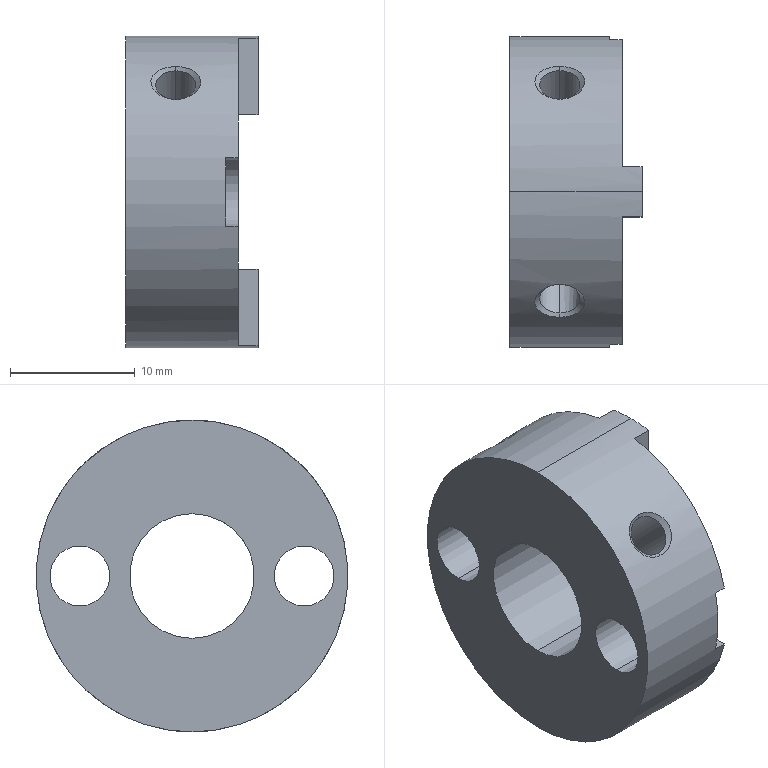Part | STEP file | _DBA11-D25-d10-e12-001.stp | 1 solid | 47 faces | box 10.6 x 25 x 25 mm | volume 3291 mm3 | cylinder 21 | plane 14 | cone 12 | commonest cylinder face diameters 2.013 x4 3.242 x4 4.8 x4 13 x3 5.58 x2 10 x2